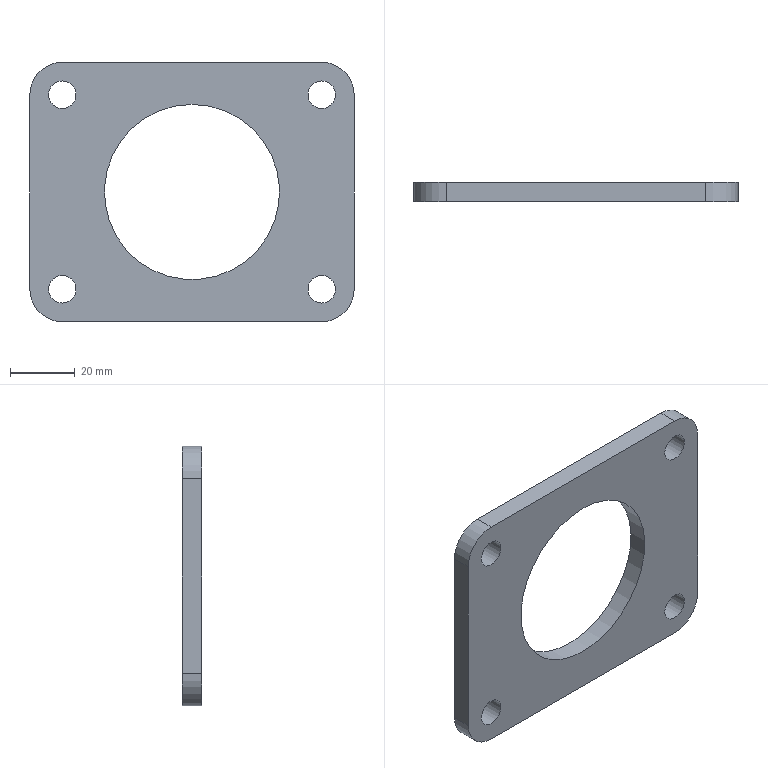Part | STEP file | JBJ-P-1017-01 | 1 solid | 15 faces | box 100 x 6 x 80 mm | volume 32382 mm3 | cylinder 9 | plane 6 | commonest cylinder face diameters 8.5 x4 20 x4 54 x1
STEP:
#1=CARTESIAN_POINT('',(-40.,6.,-25.75));
#2=VERTEX_POINT('',#1);
#3=CARTESIAN_POINT('',(-40.,6.,-30.));
#4=DIRECTION('',(0.,1.,0.));
#5=DIRECTION('',(0.,0.,1.));
#6=AXIS2_PLACEMENT_3D('',#3,#4,#5);
#7=CIRCLE('',#6,4.25);
#8=EDGE_CURVE('',#2,#2,#7,.T.);
#9=ORIENTED_EDGE('',*,*,#8,.F.);
#10=EDGE_LOOP('',(#9));
#11=FACE_BOUND('',#10,.T.);
#12=CARTESIAN_POINT('',(40.,6.,-25.75));
#13=VERTEX_POINT('',#12);
#14=CARTESIAN_POINT('',(40.,6.,-30.));
#15=DIRECTION('',(0.,1.,0.));
#16=DIRECTION('',(0.,0.,1.));
#17=AXIS2_PLACEMENT_3D('',#14,#15,#16);
#18=CIRCLE('',#17,4.25);
#19=EDGE_CURVE('',#13,#13,#18,.T.);
#20=ORIENTED_EDGE('',*,*,#19,.F.);
#21=EDGE_LOOP('',(#20));
#22=FACE_BOUND('',#21,.T.);
#23=CARTESIAN_POINT('',(40.,6.,34.25));
#24=VERTEX_POINT('',#23);
#25=CARTESIAN_POINT('',(40.,6.,30.));
#26=DIRECTION('',(0.,1.,0.));
#27=DIRECTION('',(0.,0.,1.));
#28=AXIS2_PLACEMENT_3D('',#25,#26,#27);
#29=CIRCLE('',#28,4.25);
#30=EDGE_CURVE('',#24,#24,#29,.T.);
#31=ORIENTED_EDGE('',*,*,#30,.F.);
#32=EDGE_LOOP('',(#31));
#33=FACE_BOUND('',#32,.T.);
#34=CARTESIAN_POINT('',(-40.,6.,34.25));
#35=VERTEX_POINT('',#34);
#36=CARTESIAN_POINT('',(-40.,6.,30.));
#37=DIRECTION('',(0.,1.,0.));
#38=DIRECTION('',(0.,0.,1.));
#39=AXIS2_PLACEMENT_3D('',#36,#37,#38);
#40=CIRCLE('',#39,4.25);
#41=EDGE_CURVE('',#35,#35,#40,.T.);
#42=ORIENTED_EDGE('',*,*,#41,.F.);
#43=EDGE_LOOP('',(#42));
#44=FACE_BOUND('',#43,.T.);
#45=CARTESIAN_POINT('',(-40.,6.,40.));
#46=VERTEX_POINT('',#45);
#47=CARTESIAN_POINT('',(40.,6.,40.));
#48=VERTEX_POINT('',#47);
#49=CARTESIAN_POINT('',(-50.,6.,40.));
#50=DIRECTION('',(1.,0.,0.));
#51=VECTOR('',#50,1000.);
#52=LINE('',#49,#51);
#53=EDGE_CURVE('',#46,#48,#52,.T.);
#54=ORIENTED_EDGE('',*,*,#53,.T.);
#55=CARTESIAN_POINT('',(50.,6.,30.));
#56=VERTEX_POINT('',#55);
#57=CARTESIAN_POINT('',(40.,6.,30.));
#58=DIRECTION('',(0.,1.,0.));
#59=DIRECTION('',(0.,0.,1.));
#60=AXIS2_PLACEMENT_3D('',#57,#58,#59);
#61=CIRCLE('',#60,10.);
#62=EDGE_CURVE('',#48,#56,#61,.T.);
#63=ORIENTED_EDGE('',*,*,#62,.T.);
#64=CARTESIAN_POINT('',(50.,6.,-30.));
#65=VERTEX_POINT('',#64);
#66=CARTESIAN_POINT('',(50.,6.,-40.));
#67=DIRECTION('',(0.,0.,-1.));
#68=VECTOR('',#67,1000.);
#69=LINE('',#66,#68);
#70=EDGE_CURVE('',#56,#65,#69,.T.);
#71=ORIENTED_EDGE('',*,*,#70,.T.);
#72=CARTESIAN_POINT('',(40.,6.,-40.));
#73=VERTEX_POINT('',#72);
#74=CARTESIAN_POINT('',(40.,6.,-30.));
#75=DIRECTION('',(0.,1.,0.));
#76=DIRECTION('',(0.,0.,1.));
#77=AXIS2_PLACEMENT_3D('',#74,#75,#76);
#78=CIRCLE('',#77,10.);
#79=EDGE_CURVE('',#65,#73,#78,.T.);
#80=ORIENTED_EDGE('',*,*,#79,.T.);
#81=CARTESIAN_POINT('',(-40.,6.,-40.));
#82=VERTEX_POINT('',#81);
#83=CARTESIAN_POINT('',(-50.,6.,-40.));
#84=DIRECTION('',(-1.,0.,0.));
#85=VECTOR('',#84,1000.);
#86=LINE('',#83,#85);
#87=EDGE_CURVE('',#73,#82,#86,.T.);
#88=ORIENTED_EDGE('',*,*,#87,.T.);
#89=CARTESIAN_POINT('',(-50.,6.,-30.));
#90=VERTEX_POINT('',#89);
#91=CARTESIAN_POINT('',(-40.,6.,-30.));
#92=DIRECTION('',(0.,1.,0.));
#93=DIRECTION('',(0.,0.,1.));
#94=AXIS2_PLACEMENT_3D('',#91,#92,#93);
#95=CIRCLE('',#94,10.);
#96=EDGE_CURVE('',#82,#90,#95,.T.);
#97=ORIENTED_EDGE('',*,*,#96,.T.);
#98=CARTESIAN_POINT('',(-50.,6.,30.));
#99=VERTEX_POINT('',#98);
#100=CARTESIAN_POINT('',(-50.,6.,-40.));
#101=DIRECTION('',(0.,0.,1.));
#102=VECTOR('',#101,1000.);
#103=LINE('',#100,#102);
#104=EDGE_CURVE('',#90,#99,#103,.T.);
#105=ORIENTED_EDGE('',*,*,#104,.T.);
#106=CARTESIAN_POINT('',(-40.,6.,30.));
#107=DIRECTION('',(0.,1.,0.));
#108=DIRECTION('',(0.,0.,1.));
#109=AXIS2_PLACEMENT_3D('',#106,#107,#108);
#110=CIRCLE('',#109,10.);
#111=EDGE_CURVE('',#99,#46,#110,.T.);
#112=ORIENTED_EDGE('',*,*,#111,.T.);
#113=EDGE_LOOP('',(#54,#63,#71,#80,#88,#97,#105,#112));
#114=FACE_OUTER_BOUND('',#113,.T.);
#115=CARTESIAN_POINT('',(0.,6.,27.));
#116=VERTEX_POINT('',#115);
#117=CARTESIAN_POINT('',(0.,6.,0.));
#118=DIRECTION('',(0.,1.,0.));
#119=DIRECTION('',(0.,0.,1.));
#120=AXIS2_PLACEMENT_3D('',#117,#118,#119);
#121=CIRCLE('',#120,27.);
#122=EDGE_CURVE('',#116,#116,#121,.T.);
#123=ORIENTED_EDGE('',*,*,#122,.F.);
#124=EDGE_LOOP('',(#123));
#125=FACE_BOUND('',#124,.T.);
#126=CARTESIAN_POINT('',(0.,6.,0.));
#127=DIRECTION('',(0.,1.,0.));
#128=DIRECTION('',(0.,0.,1.));
#129=AXIS2_PLACEMENT_3D('',#126,#127,#128);
#130=PLANE('',#129);
#131=ADVANCED_FACE('',(#11,#22,#33,#44,#114,#125),#130,.T.);
#132=CARTESIAN_POINT('',(-40.,0.,-25.75));
#133=VERTEX_POINT('',#132);
#134=CARTESIAN_POINT('',(-40.,0.,-30.));
#135=DIRECTION('',(0.,1.,0.));
#136=DIRECTION('',(0.,0.,1.));
#137=AXIS2_PLACEMENT_3D('',#134,#135,#136);
#138=CIRCLE('',#137,4.25);
#139=EDGE_CURVE('',#133,#133,#138,.T.);
#140=ORIENTED_EDGE('',*,*,#139,.T.);
#141=EDGE_LOOP('',(#140));
#142=FACE_BOUND('',#141,.T.);
#143=CARTESIAN_POINT('',(40.,0.,-25.75));
#144=VERTEX_POINT('',#143);
#145=CARTESIAN_POINT('',(40.,0.,-30.));
#146=DIRECTION('',(0.,1.,0.));
#147=DIRECTION('',(0.,0.,1.));
#148=AXIS2_PLACEMENT_3D('',#145,#146,#147);
#149=CIRCLE('',#148,4.25);
#150=EDGE_CURVE('',#144,#144,#149,.T.);
#151=ORIENTED_EDGE('',*,*,#150,.T.);
#152=EDGE_LOOP('',(#151));
#153=FACE_BOUND('',#152,.T.);
#154=CARTESIAN_POINT('',(40.,0.,34.25));
#155=VERTEX_POINT('',#154);
#156=CARTESIAN_POINT('',(40.,0.,30.));
#157=DIRECTION('',(0.,1.,0.));
#158=DIRECTION('',(0.,0.,1.));
#159=AXIS2_PLACEMENT_3D('',#156,#157,#158);
#160=CIRCLE('',#159,4.25);
#161=EDGE_CURVE('',#155,#155,#160,.T.);
#162=ORIENTED_EDGE('',*,*,#161,.T.);
#163=EDGE_LOOP('',(#162));
#164=FACE_BOUND('',#163,.T.);
#165=CARTESIAN_POINT('',(-40.,0.,34.25));
#166=VERTEX_POINT('',#165);
#167=CARTESIAN_POINT('',(-40.,0.,30.));
#168=DIRECTION('',(0.,1.,0.));
#169=DIRECTION('',(0.,0.,1.));
#170=AXIS2_PLACEMENT_3D('',#167,#168,#169);
#171=CIRCLE('',#170,4.25);
#172=EDGE_CURVE('',#166,#166,#171,.T.);
#173=ORIENTED_EDGE('',*,*,#172,.T.);
#174=EDGE_LOOP('',(#173));
#175=FACE_BOUND('',#174,.T.);
#176=CARTESIAN_POINT('',(50.,0.,30.));
#177=VERTEX_POINT('',#176);
#178=CARTESIAN_POINT('',(50.,0.,-30.));
#179=VERTEX_POINT('',#178);
#180=CARTESIAN_POINT('',(50.,0.,-40.));
#181=DIRECTION('',(0.,0.,-1.));
#182=VECTOR('',#181,1000.);
#183=LINE('',#180,#182);
#184=EDGE_CURVE('',#177,#179,#183,.T.);
#185=ORIENTED_EDGE('',*,*,#184,.F.);
#186=CARTESIAN_POINT('',(40.,0.,40.));
#187=VERTEX_POINT('',#186);
#188=CARTESIAN_POINT('',(40.,0.,30.));
#189=DIRECTION('',(0.,-1.,0.));
#190=DIRECTION('',(0.,0.,1.));
#191=AXIS2_PLACEMENT_3D('',#188,#189,#190);
#192=CIRCLE('',#191,10.);
#193=EDGE_CURVE('',#177,#187,#192,.T.);
#194=ORIENTED_EDGE('',*,*,#193,.T.);
#195=CARTESIAN_POINT('',(-40.,0.,40.));
#196=VERTEX_POINT('',#195);
#197=CARTESIAN_POINT('',(-50.,0.,40.));
#198=DIRECTION('',(1.,0.,0.));
#199=VECTOR('',#198,1000.);
#200=LINE('',#197,#199);
#201=EDGE_CURVE('',#196,#187,#200,.T.);
#202=ORIENTED_EDGE('',*,*,#201,.F.);
#203=CARTESIAN_POINT('',(-50.,0.,30.));
#204=VERTEX_POINT('',#203);
#205=CARTESIAN_POINT('',(-40.,0.,30.));
#206=DIRECTION('',(0.,-1.,0.));
#207=DIRECTION('',(0.,0.,1.));
#208=AXIS2_PLACEMENT_3D('',#205,#206,#207);
#209=CIRCLE('',#208,10.);
#210=EDGE_CURVE('',#196,#204,#209,.T.);
#211=ORIENTED_EDGE('',*,*,#210,.T.);
#212=CARTESIAN_POINT('',(-50.,0.,-30.));
#213=VERTEX_POINT('',#212);
#214=CARTESIAN_POINT('',(-50.,0.,-40.));
#215=DIRECTION('',(0.,0.,1.));
#216=VECTOR('',#215,1000.);
#217=LINE('',#214,#216);
#218=EDGE_CURVE('',#213,#204,#217,.T.);
#219=ORIENTED_EDGE('',*,*,#218,.F.);
#220=CARTESIAN_POINT('',(-40.,0.,-40.));
#221=VERTEX_POINT('',#220);
#222=CARTESIAN_POINT('',(-40.,0.,-30.));
#223=DIRECTION('',(0.,-1.,0.));
#224=DIRECTION('',(0.,0.,1.));
#225=AXIS2_PLACEMENT_3D('',#222,#223,#224);
#226=CIRCLE('',#225,10.);
#227=EDGE_CURVE('',#213,#221,#226,.T.);
#228=ORIENTED_EDGE('',*,*,#227,.T.);
#229=CARTESIAN_POINT('',(40.,0.,-40.));
#230=VERTEX_POINT('',#229);
#231=CARTESIAN_POINT('',(-50.,0.,-40.));
#232=DIRECTION('',(-1.,0.,0.));
#233=VECTOR('',#232,1000.);
#234=LINE('',#231,#233);
#235=EDGE_CURVE('',#230,#221,#234,.T.);
#236=ORIENTED_EDGE('',*,*,#235,.F.);
#237=CARTESIAN_POINT('',(40.,0.,-30.));
#238=DIRECTION('',(0.,-1.,0.));
#239=DIRECTION('',(0.,0.,1.));
#240=AXIS2_PLACEMENT_3D('',#237,#238,#239);
#241=CIRCLE('',#240,10.);
#242=EDGE_CURVE('',#230,#179,#241,.T.);
#243=ORIENTED_EDGE('',*,*,#242,.T.);
#244=EDGE_LOOP('',(#185,#194,#202,#211,#219,#228,#236,#243));
#245=FACE_OUTER_BOUND('',#244,.T.);
#246=CARTESIAN_POINT('',(0.,0.,27.));
#247=VERTEX_POINT('',#246);
#248=CARTESIAN_POINT('',(0.,0.,0.));
#249=DIRECTION('',(0.,1.,0.));
#250=DIRECTION('',(0.,0.,1.));
#251=AXIS2_PLACEMENT_3D('',#248,#249,#250);
#252=CIRCLE('',#251,27.);
#253=EDGE_CURVE('',#247,#247,#252,.T.);
#254=ORIENTED_EDGE('',*,*,#253,.T.);
#255=EDGE_LOOP('',(#254));
#256=FACE_BOUND('',#255,.T.);
#257=CARTESIAN_POINT('',(0.,0.,0.));
#258=DIRECTION('',(0.,1.,0.));
#259=DIRECTION('',(0.,0.,1.));
#260=AXIS2_PLACEMENT_3D('',#257,#258,#259);
#261=PLANE('',#260);
#262=ADVANCED_FACE('',(#142,#153,#164,#175,#245,#256),#261,.F.);
#263=ORIENTED_EDGE('',*,*,#70,.F.);
#264=CARTESIAN_POINT('',(50.,6.,30.));
#265=DIRECTION('',(0.,-1.,0.));
#266=VECTOR('',#265,1000.);
#267=LINE('',#264,#266);
#268=EDGE_CURVE('',#56,#177,#267,.T.);
#269=ORIENTED_EDGE('',*,*,#268,.T.);
#270=ORIENTED_EDGE('',*,*,#184,.T.);
#271=CARTESIAN_POINT('',(50.,6.,-30.));
#272=DIRECTION('',(0.,1.,0.));
#273=VECTOR('',#272,1000.);
#274=LINE('',#271,#273);
#275=EDGE_CURVE('',#179,#65,#274,.T.);
#276=ORIENTED_EDGE('',*,*,#275,.T.);
#277=EDGE_LOOP('',(#263,#269,#270,#276));
#278=FACE_OUTER_BOUND('',#277,.T.);
#279=CARTESIAN_POINT('',(50.,6.,-40.));
#280=DIRECTION('',(-1.,0.,0.));
#281=DIRECTION('',(0.,0.,1.));
#282=AXIS2_PLACEMENT_3D('',#279,#280,#281);
#283=PLANE('',#282);
#284=ADVANCED_FACE('',(#278),#283,.F.);
#285=ORIENTED_EDGE('',*,*,#87,.F.);
#286=CARTESIAN_POINT('',(40.,6.,-40.));
#287=DIRECTION('',(0.,-1.,0.));
#288=VECTOR('',#287,1000.);
#289=LINE('',#286,#288);
#290=EDGE_CURVE('',#73,#230,#289,.T.);
#291=ORIENTED_EDGE('',*,*,#290,.T.);
#292=ORIENTED_EDGE('',*,*,#235,.T.);
#293=CARTESIAN_POINT('',(-40.,6.,-40.));
#294=DIRECTION('',(0.,1.,0.));
#295=VECTOR('',#294,1000.);
#296=LINE('',#293,#295);
#297=EDGE_CURVE('',#221,#82,#296,.T.);
#298=ORIENTED_EDGE('',*,*,#297,.T.);
#299=EDGE_LOOP('',(#285,#291,#292,#298));
#300=FACE_OUTER_BOUND('',#299,.T.);
#301=CARTESIAN_POINT('',(-50.,6.,-40.));
#302=DIRECTION('',(0.,0.,1.));
#303=DIRECTION('',(1.,0.,0.));
#304=AXIS2_PLACEMENT_3D('',#301,#302,#303);
#305=PLANE('',#304);
#306=ADVANCED_FACE('',(#300),#305,.F.);
#307=ORIENTED_EDGE('',*,*,#104,.F.);
#308=CARTESIAN_POINT('',(-50.,6.,-30.));
#309=DIRECTION('',(0.,-1.,0.));
#310=VECTOR('',#309,1000.);
#311=LINE('',#308,#310);
#312=EDGE_CURVE('',#90,#213,#311,.T.);
#313=ORIENTED_EDGE('',*,*,#312,.T.);
#314=ORIENTED_EDGE('',*,*,#218,.T.);
#315=CARTESIAN_POINT('',(-50.,6.,30.));
#316=DIRECTION('',(0.,1.,0.));
#317=VECTOR('',#316,1000.);
#318=LINE('',#315,#317);
#319=EDGE_CURVE('',#204,#99,#318,.T.);
#320=ORIENTED_EDGE('',*,*,#319,.T.);
#321=EDGE_LOOP('',(#307,#313,#314,#320));
#322=FACE_OUTER_BOUND('',#321,.T.);
#323=CARTESIAN_POINT('',(-50.,6.,-40.));
#324=DIRECTION('',(1.,0.,0.));
#325=DIRECTION('',(0.,0.,-1.));
#326=AXIS2_PLACEMENT_3D('',#323,#324,#325);
#327=PLANE('',#326);
#328=ADVANCED_FACE('',(#322),#327,.F.);
#329=ORIENTED_EDGE('',*,*,#201,.T.);
#330=CARTESIAN_POINT('',(40.,6.,40.));
#331=DIRECTION('',(0.,1.,0.));
#332=VECTOR('',#331,1000.);
#333=LINE('',#330,#332);
#334=EDGE_CURVE('',#187,#48,#333,.T.);
#335=ORIENTED_EDGE('',*,*,#334,.T.);
#336=ORIENTED_EDGE('',*,*,#53,.F.);
#337=CARTESIAN_POINT('',(-40.,6.,40.));
#338=DIRECTION('',(0.,-1.,0.));
#339=VECTOR('',#338,1000.);
#340=LINE('',#337,#339);
#341=EDGE_CURVE('',#46,#196,#340,.T.);
#342=ORIENTED_EDGE('',*,*,#341,.T.);
#343=EDGE_LOOP('',(#329,#335,#336,#342));
#344=FACE_OUTER_BOUND('',#343,.T.);
#345=CARTESIAN_POINT('',(-50.,6.,40.));
#346=DIRECTION('',(0.,0.,-1.));
#347=DIRECTION('',(-1.,0.,0.));
#348=AXIS2_PLACEMENT_3D('',#345,#346,#347);
#349=PLANE('',#348);
#350=ADVANCED_FACE('',(#344),#349,.F.);
#351=ORIENTED_EDGE('',*,*,#122,.T.);
#352=EDGE_LOOP('',(#351));
#353=FACE_OUTER_BOUND('',#352,.T.);
#354=ORIENTED_EDGE('',*,*,#253,.F.);
#355=EDGE_LOOP('',(#354));
#356=FACE_OUTER_BOUND('',#355,.T.);
#357=CARTESIAN_POINT('',(0.,6.,0.));
#358=DIRECTION('',(0.,-1.,0.));
#359=DIRECTION('',(0.,0.,-1.));
#360=AXIS2_PLACEMENT_3D('',#357,#358,#359);
#361=CYLINDRICAL_SURFACE('',#360,27.);
#362=ADVANCED_FACE('',(#353,#356),#361,.F.);
#363=ORIENTED_EDGE('',*,*,#62,.F.);
#364=ORIENTED_EDGE('',*,*,#334,.F.);
#365=ORIENTED_EDGE('',*,*,#193,.F.);
#366=ORIENTED_EDGE('',*,*,#268,.F.);
#367=EDGE_LOOP('',(#363,#364,#365,#366));
#368=FACE_OUTER_BOUND('',#367,.T.);
#369=CARTESIAN_POINT('',(40.,6.,30.));
#370=DIRECTION('',(0.,-1.,0.));
#371=DIRECTION('',(0.,0.,-1.));
#372=AXIS2_PLACEMENT_3D('',#369,#370,#371);
#373=CYLINDRICAL_SURFACE('',#372,10.);
#374=ADVANCED_FACE('',(#368),#373,.T.);
#375=ORIENTED_EDGE('',*,*,#79,.F.);
#376=ORIENTED_EDGE('',*,*,#275,.F.);
#377=ORIENTED_EDGE('',*,*,#242,.F.);
#378=ORIENTED_EDGE('',*,*,#290,.F.);
#379=EDGE_LOOP('',(#375,#376,#377,#378));
#380=FACE_OUTER_BOUND('',#379,.T.);
#381=CARTESIAN_POINT('',(40.,6.,-30.));
#382=DIRECTION('',(0.,-1.,0.));
#383=DIRECTION('',(0.,0.,-1.));
#384=AXIS2_PLACEMENT_3D('',#381,#382,#383);
#385=CYLINDRICAL_SURFACE('',#384,10.);
#386=ADVANCED_FACE('',(#380),#385,.T.);
#387=ORIENTED_EDGE('',*,*,#96,.F.);
#388=ORIENTED_EDGE('',*,*,#297,.F.);
#389=ORIENTED_EDGE('',*,*,#227,.F.);
#390=ORIENTED_EDGE('',*,*,#312,.F.);
#391=EDGE_LOOP('',(#387,#388,#389,#390));
#392=FACE_OUTER_BOUND('',#391,.T.);
#393=CARTESIAN_POINT('',(-40.,6.,-30.));
#394=DIRECTION('',(0.,-1.,0.));
#395=DIRECTION('',(0.,0.,-1.));
#396=AXIS2_PLACEMENT_3D('',#393,#394,#395);
#397=CYLINDRICAL_SURFACE('',#396,10.);
#398=ADVANCED_FACE('',(#392),#397,.T.);
#399=ORIENTED_EDGE('',*,*,#111,.F.);
#400=ORIENTED_EDGE('',*,*,#319,.F.);
#401=ORIENTED_EDGE('',*,*,#210,.F.);
#402=ORIENTED_EDGE('',*,*,#341,.F.);
#403=EDGE_LOOP('',(#399,#400,#401,#402));
#404=FACE_OUTER_BOUND('',#403,.T.);
#405=CARTESIAN_POINT('',(-40.,6.,30.));
#406=DIRECTION('',(0.,-1.,0.));
#407=DIRECTION('',(0.,0.,-1.));
#408=AXIS2_PLACEMENT_3D('',#405,#406,#407);
#409=CYLINDRICAL_SURFACE('',#408,10.);
#410=ADVANCED_FACE('',(#404),#409,.T.);
#411=ORIENTED_EDGE('',*,*,#172,.F.);
#412=EDGE_LOOP('',(#411));
#413=FACE_OUTER_BOUND('',#412,.T.);
#414=ORIENTED_EDGE('',*,*,#41,.T.);
#415=EDGE_LOOP('',(#414));
#416=FACE_OUTER_BOUND('',#415,.T.);
#417=CARTESIAN_POINT('',(-40.,6.,30.));
#418=DIRECTION('',(0.,1.,0.));
#419=DIRECTION('',(0.,0.,1.));
#420=AXIS2_PLACEMENT_3D('',#417,#418,#419);
#421=CYLINDRICAL_SURFACE('',#420,4.25);
#422=ADVANCED_FACE('',(#413,#416),#421,.F.);
#423=ORIENTED_EDGE('',*,*,#161,.F.);
#424=EDGE_LOOP('',(#423));
#425=FACE_OUTER_BOUND('',#424,.T.);
#426=ORIENTED_EDGE('',*,*,#30,.T.);
#427=EDGE_LOOP('',(#426));
#428=FACE_OUTER_BOUND('',#427,.T.);
#429=CARTESIAN_POINT('',(40.,6.,30.));
#430=DIRECTION('',(0.,1.,0.));
#431=DIRECTION('',(0.,0.,1.));
#432=AXIS2_PLACEMENT_3D('',#429,#430,#431);
#433=CYLINDRICAL_SURFACE('',#432,4.25);
#434=ADVANCED_FACE('',(#425,#428),#433,.F.);
#435=ORIENTED_EDGE('',*,*,#150,.F.);
#436=EDGE_LOOP('',(#435));
#437=FACE_OUTER_BOUND('',#436,.T.);
#438=ORIENTED_EDGE('',*,*,#19,.T.);
#439=EDGE_LOOP('',(#438));
#440=FACE_OUTER_BOUND('',#439,.T.);
#441=CARTESIAN_POINT('',(40.,6.,-30.));
#442=DIRECTION('',(0.,1.,0.));
#443=DIRECTION('',(0.,0.,1.));
#444=AXIS2_PLACEMENT_3D('',#441,#442,#443);
#445=CYLINDRICAL_SURFACE('',#444,4.25);
#446=ADVANCED_FACE('',(#437,#440),#445,.F.);
#447=ORIENTED_EDGE('',*,*,#139,.F.);
#448=EDGE_LOOP('',(#447));
#449=FACE_OUTER_BOUND('',#448,.T.);
#450=ORIENTED_EDGE('',*,*,#8,.T.);
#451=EDGE_LOOP('',(#450));
#452=FACE_OUTER_BOUND('',#451,.T.);
#453=CARTESIAN_POINT('',(-40.,6.,-30.));
#454=DIRECTION('',(0.,1.,0.));
#455=DIRECTION('',(0.,0.,1.));
#456=AXIS2_PLACEMENT_3D('',#453,#454,#455);
#457=CYLINDRICAL_SURFACE('',#456,4.25);
#458=ADVANCED_FACE('',(#449,#452),#457,.F.);
#459=CLOSED_SHELL('',(#131,#262,#284,#306,#328,#350,#362,#374,#386,#398,#410,#422,#434,#446,#458));
#460=MANIFOLD_SOLID_BREP('',#459);
#461=CARTESIAN_POINT('',(0.,0.,0.));
#462=DIRECTION('',(0.,0.,1.));
#463=DIRECTION('',(1.,0.,0.));
#464=AXIS2_PLACEMENT_3D('',#461,#462,#463);
#465=(LENGTH_UNIT()NAMED_UNIT(*)SI_UNIT(.MILLI.,.METRE.));
#466=UNCERTAINTY_MEASURE_WITH_UNIT(LENGTH_MEASURE(0.00001),#465,'','');
#467=(NAMED_UNIT(*)PLANE_ANGLE_UNIT()SI_UNIT($,.RADIAN.));
#468=(NAMED_UNIT(*)SI_UNIT($,.STERADIAN.)SOLID_ANGLE_UNIT());
#469=(GEOMETRIC_REPRESENTATION_CONTEXT(3)GLOBAL_UNCERTAINTY_ASSIGNED_CONTEXT((#466))GLOBAL_UNIT_ASSIGNED_CONTEXT((#465,#467,#468))REPRESENTATION_CONTEXT('',''));
#470=ADVANCED_BREP_SHAPE_REPRESENTATION('',(#460,#464),#469);